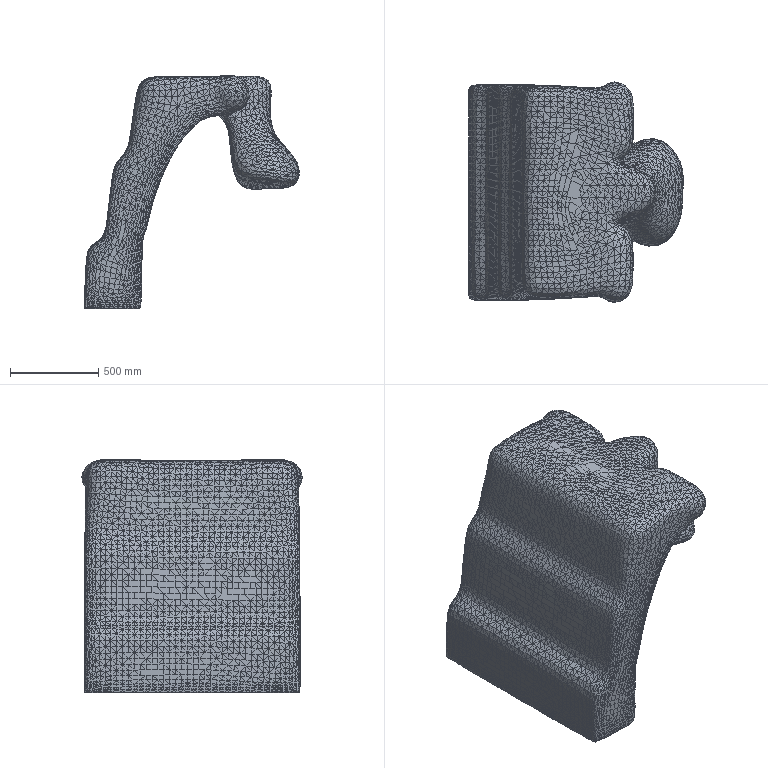Part | SolidWorks | features BaseBody 1, ICE 1, Scale 1 | 1 solid | 13769 faces | volume 395223712 mm3 | plane 13769